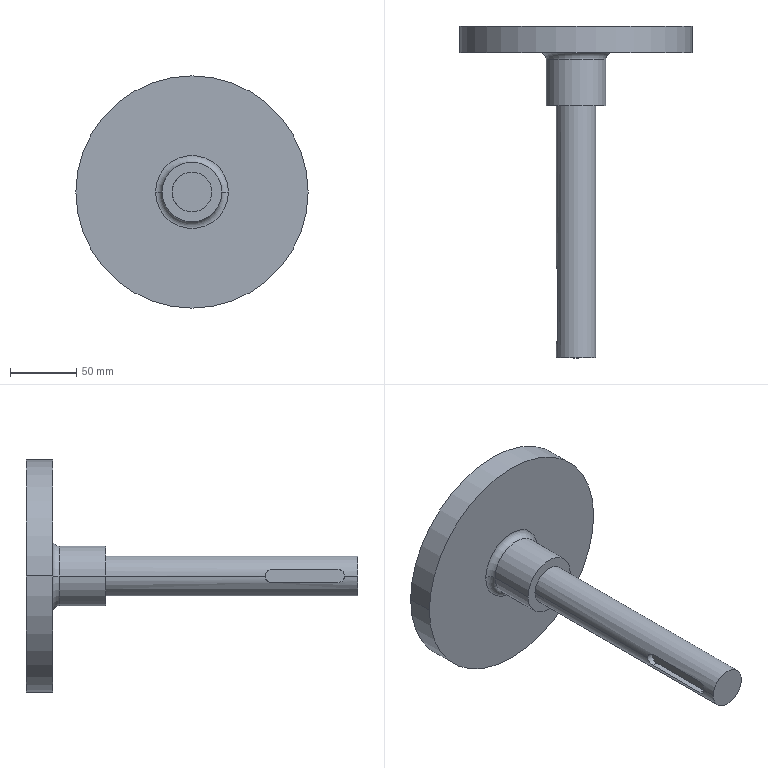Part | STEP file | Roller XG3 | 1 solid | 18 faces | box 175 x 250 x 175 mm | volume 677038 mm3 | cylinder 9 | plane 7 | torus 2 | commonest cylinder face diameters 10 x3 30 x2 45 x2 175 x2